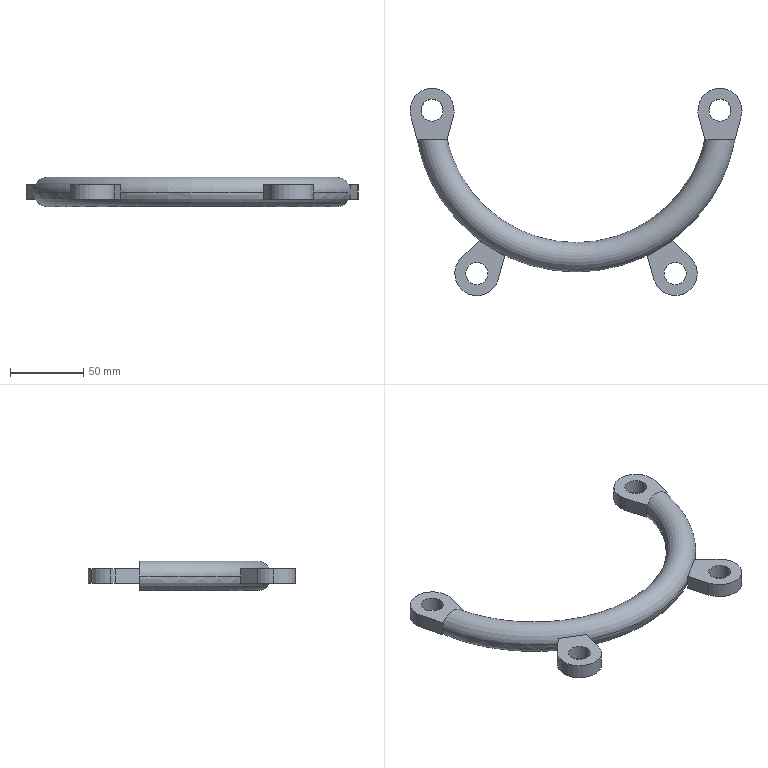Part | SolidWorks | features ICE 3, MirrorPattern 1, Sweep 1 | 3 solids | 53 faces | box 225.916 x 141.102 x 20 mm | volume 58505 mm3 | plane 32 | cylinder 17 | torus 4 | commonest cylinder face diameters 30 x9 15 x8